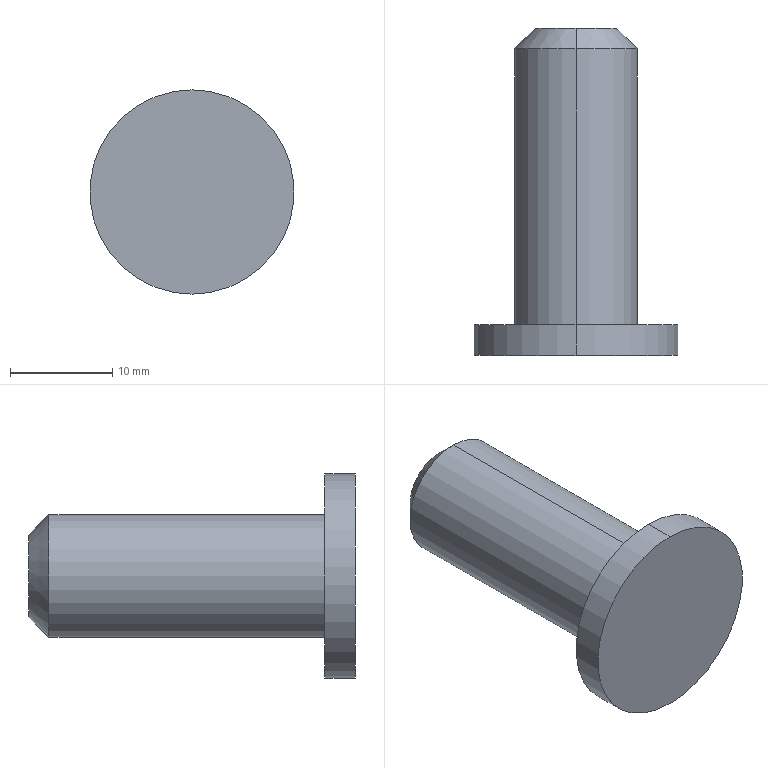Part | SolidWorks | features Chamfer 1, Revolution 1 | 1 solid | 9 faces | box 20 x 32 x 20 mm | volume 4155 mm3 | cylinder 4 | plane 3 | cone 2 | commonest cylinder face diameters 12 x2 20 x2
STEP:
#1=CARTESIAN_POINT('',(0.,32.,4.));
#2=VERTEX_POINT('',#1);
#3=CARTESIAN_POINT('',(0.,32.,-4.));
#4=VERTEX_POINT('',#3);
#5=CARTESIAN_POINT('',(0.,32.,0.));
#6=DIRECTION('',(0.,1.,0.));
#7=DIRECTION('',(0.,0.,1.));
#8=AXIS2_PLACEMENT_3D('',#5,#6,#7);
#9=CIRCLE('',#8,4.);
#10=EDGE_CURVE('',#2,#4,#9,.T.);
#11=ORIENTED_EDGE('',*,*,#10,.F.);
#12=CARTESIAN_POINT('',(0.,30.,6.));
#13=VERTEX_POINT('',#12);
#14=CARTESIAN_POINT('',(0.,30.,6.));
#15=DIRECTION('',(0.,-0.7071,0.7071));
#16=VECTOR('',#15,1000.);
#17=LINE('',#14,#16);
#18=EDGE_CURVE('',#2,#13,#17,.T.);
#19=ORIENTED_EDGE('',*,*,#18,.T.);
#20=CARTESIAN_POINT('',(0.,30.,-6.));
#21=VERTEX_POINT('',#20);
#22=CARTESIAN_POINT('',(0.,30.,0.));
#23=DIRECTION('',(0.,-1.,0.));
#24=DIRECTION('',(0.,0.,1.));
#25=AXIS2_PLACEMENT_3D('',#22,#23,#24);
#26=CIRCLE('',#25,6.);
#27=EDGE_CURVE('',#21,#13,#26,.T.);
#28=ORIENTED_EDGE('',*,*,#27,.F.);
#29=CARTESIAN_POINT('',(0.,30.,-6.));
#30=DIRECTION('',(0.,-0.7071,-0.7071));
#31=VECTOR('',#30,1000.);
#32=LINE('',#29,#31);
#33=EDGE_CURVE('',#4,#21,#32,.T.);
#34=ORIENTED_EDGE('',*,*,#33,.F.);
#35=EDGE_LOOP('',(#11,#19,#28,#34));
#36=FACE_OUTER_BOUND('',#35,.T.);
#37=CARTESIAN_POINT('',(0.,30.,0.));
#38=DIRECTION('',(0.,-1.,0.));
#39=DIRECTION('',(0.,0.,-1.));
#40=AXIS2_PLACEMENT_3D('',#37,#38,#39);
#41=CONICAL_SURFACE('',#40,6.,0.7854);
#42=ADVANCED_FACE('',(#36),#41,.T.);
#43=ORIENTED_EDGE('',*,*,#27,.T.);
#44=CARTESIAN_POINT('',(0.,3.,6.));
#45=VERTEX_POINT('',#44);
#46=CARTESIAN_POINT('',(0.,0.,6.));
#47=DIRECTION('',(0.,-1.,0.));
#48=VECTOR('',#47,1000.);
#49=LINE('',#46,#48);
#50=EDGE_CURVE('',#13,#45,#49,.T.);
#51=ORIENTED_EDGE('',*,*,#50,.T.);
#52=CARTESIAN_POINT('',(0.,3.,-6.));
#53=VERTEX_POINT('',#52);
#54=CARTESIAN_POINT('',(0.,3.,0.));
#55=DIRECTION('',(0.,-1.,0.));
#56=DIRECTION('',(0.,0.,-1.));
#57=AXIS2_PLACEMENT_3D('',#54,#55,#56);
#58=CIRCLE('',#57,6.);
#59=EDGE_CURVE('',#53,#45,#58,.T.);
#60=ORIENTED_EDGE('',*,*,#59,.F.);
#61=CARTESIAN_POINT('',(0.,0.,-6.));
#62=DIRECTION('',(0.,-1.,0.));
#63=VECTOR('',#62,1000.);
#64=LINE('',#61,#63);
#65=EDGE_CURVE('',#21,#53,#64,.T.);
#66=ORIENTED_EDGE('',*,*,#65,.F.);
#67=EDGE_LOOP('',(#43,#51,#60,#66));
#68=FACE_OUTER_BOUND('',#67,.T.);
#69=CARTESIAN_POINT('',(0.,0.,0.));
#70=DIRECTION('',(0.,-1.,0.));
#71=DIRECTION('',(0.,0.,-1.));
#72=AXIS2_PLACEMENT_3D('',#69,#70,#71);
#73=CYLINDRICAL_SURFACE('',#72,6.);
#74=ADVANCED_FACE('',(#68),#73,.T.);
#75=CARTESIAN_POINT('',(0.,3.,-10.));
#76=VERTEX_POINT('',#75);
#77=CARTESIAN_POINT('',(0.,3.,10.));
#78=VERTEX_POINT('',#77);
#79=CARTESIAN_POINT('',(0.,3.,0.));
#80=DIRECTION('',(0.,-1.,0.));
#81=DIRECTION('',(0.,0.,-1.));
#82=AXIS2_PLACEMENT_3D('',#79,#80,#81);
#83=CIRCLE('',#82,10.);
#84=EDGE_CURVE('',#76,#78,#83,.T.);
#85=ORIENTED_EDGE('',*,*,#84,.T.);
#86=CARTESIAN_POINT('',(0.,0.,10.));
#87=VERTEX_POINT('',#86);
#88=CARTESIAN_POINT('',(0.,0.,10.));
#89=DIRECTION('',(0.,-1.,0.));
#90=VECTOR('',#89,1000.);
#91=LINE('',#88,#90);
#92=EDGE_CURVE('',#78,#87,#91,.T.);
#93=ORIENTED_EDGE('',*,*,#92,.T.);
#94=CARTESIAN_POINT('',(0.,0.,-10.));
#95=VERTEX_POINT('',#94);
#96=CARTESIAN_POINT('',(0.,0.,0.));
#97=DIRECTION('',(0.,-1.,0.));
#98=DIRECTION('',(0.,0.,-1.));
#99=AXIS2_PLACEMENT_3D('',#96,#97,#98);
#100=CIRCLE('',#99,10.);
#101=EDGE_CURVE('',#95,#87,#100,.T.);
#102=ORIENTED_EDGE('',*,*,#101,.F.);
#103=CARTESIAN_POINT('',(0.,0.,-10.));
#104=DIRECTION('',(0.,-1.,0.));
#105=VECTOR('',#104,1000.);
#106=LINE('',#103,#105);
#107=EDGE_CURVE('',#76,#95,#106,.T.);
#108=ORIENTED_EDGE('',*,*,#107,.F.);
#109=EDGE_LOOP('',(#85,#93,#102,#108));
#110=FACE_OUTER_BOUND('',#109,.T.);
#111=CARTESIAN_POINT('',(0.,0.,0.));
#112=DIRECTION('',(0.,-1.,0.));
#113=DIRECTION('',(0.,0.,-1.));
#114=AXIS2_PLACEMENT_3D('',#111,#112,#113);
#115=CYLINDRICAL_SURFACE('',#114,10.);
#116=ADVANCED_FACE('',(#110),#115,.T.);
#117=ORIENTED_EDGE('',*,*,#101,.T.);
#118=CARTESIAN_POINT('',(0.,0.,0.));
#119=DIRECTION('',(0.,-1.,0.));
#120=DIRECTION('',(0.,0.,-1.));
#121=AXIS2_PLACEMENT_3D('',#118,#119,#120);
#122=CIRCLE('',#121,10.);
#123=EDGE_CURVE('',#87,#95,#122,.T.);
#124=ORIENTED_EDGE('',*,*,#123,.T.);
#125=EDGE_LOOP('',(#117,#124));
#126=FACE_OUTER_BOUND('',#125,.T.);
#127=CARTESIAN_POINT('',(0.,0.,0.));
#128=DIRECTION('',(0.,-1.,0.));
#129=DIRECTION('',(0.,0.,-1.));
#130=AXIS2_PLACEMENT_3D('',#127,#128,#129);
#131=PLANE('',#130);
#132=ADVANCED_FACE('',(#126),#131,.T.);
#133=ORIENTED_EDGE('',*,*,#92,.F.);
#134=CARTESIAN_POINT('',(0.,3.,0.));
#135=DIRECTION('',(0.,-1.,0.));
#136=DIRECTION('',(0.,0.,-1.));
#137=AXIS2_PLACEMENT_3D('',#134,#135,#136);
#138=CIRCLE('',#137,10.);
#139=EDGE_CURVE('',#78,#76,#138,.T.);
#140=ORIENTED_EDGE('',*,*,#139,.T.);
#141=ORIENTED_EDGE('',*,*,#107,.T.);
#142=ORIENTED_EDGE('',*,*,#123,.F.);
#143=EDGE_LOOP('',(#133,#140,#141,#142));
#144=FACE_OUTER_BOUND('',#143,.T.);
#145=CARTESIAN_POINT('',(0.,0.,0.));
#146=DIRECTION('',(0.,-1.,0.));
#147=DIRECTION('',(0.,0.,-1.));
#148=AXIS2_PLACEMENT_3D('',#145,#146,#147);
#149=CYLINDRICAL_SURFACE('',#148,10.);
#150=ADVANCED_FACE('',(#144),#149,.T.);
#151=ORIENTED_EDGE('',*,*,#59,.T.);
#152=CARTESIAN_POINT('',(0.,3.,0.));
#153=DIRECTION('',(0.,-1.,0.));
#154=DIRECTION('',(0.,0.,-1.));
#155=AXIS2_PLACEMENT_3D('',#152,#153,#154);
#156=CIRCLE('',#155,6.);
#157=EDGE_CURVE('',#45,#53,#156,.T.);
#158=ORIENTED_EDGE('',*,*,#157,.T.);
#159=EDGE_LOOP('',(#151,#158));
#160=FACE_BOUND('',#159,.T.);
#161=ORIENTED_EDGE('',*,*,#84,.F.);
#162=ORIENTED_EDGE('',*,*,#139,.F.);
#163=EDGE_LOOP('',(#161,#162));
#164=FACE_OUTER_BOUND('',#163,.T.);
#165=CARTESIAN_POINT('',(10.,3.,0.));
#166=DIRECTION('',(0.,1.,0.));
#167=DIRECTION('',(0.,0.,1.));
#168=AXIS2_PLACEMENT_3D('',#165,#166,#167);
#169=PLANE('',#168);
#170=ADVANCED_FACE('',(#160,#164),#169,.T.);
#171=ORIENTED_EDGE('',*,*,#50,.F.);
#172=CARTESIAN_POINT('',(0.,30.,0.));
#173=DIRECTION('',(0.,-1.,0.));
#174=DIRECTION('',(0.,0.,1.));
#175=AXIS2_PLACEMENT_3D('',#172,#173,#174);
#176=CIRCLE('',#175,6.);
#177=EDGE_CURVE('',#13,#21,#176,.T.);
#178=ORIENTED_EDGE('',*,*,#177,.T.);
#179=ORIENTED_EDGE('',*,*,#65,.T.);
#180=ORIENTED_EDGE('',*,*,#157,.F.);
#181=EDGE_LOOP('',(#171,#178,#179,#180));
#182=FACE_OUTER_BOUND('',#181,.T.);
#183=CARTESIAN_POINT('',(0.,0.,0.));
#184=DIRECTION('',(0.,-1.,0.));
#185=DIRECTION('',(0.,0.,-1.));
#186=AXIS2_PLACEMENT_3D('',#183,#184,#185);
#187=CYLINDRICAL_SURFACE('',#186,6.);
#188=ADVANCED_FACE('',(#182),#187,.T.);
#189=CARTESIAN_POINT('',(0.,32.,0.));
#190=DIRECTION('',(0.,1.,0.));
#191=DIRECTION('',(0.,0.,1.));
#192=AXIS2_PLACEMENT_3D('',#189,#190,#191);
#193=CIRCLE('',#192,4.);
#194=EDGE_CURVE('',#4,#2,#193,.T.);
#195=ORIENTED_EDGE('',*,*,#194,.T.);
#196=ORIENTED_EDGE('',*,*,#10,.T.);
#197=EDGE_LOOP('',(#195,#196));
#198=FACE_OUTER_BOUND('',#197,.T.);
#199=CARTESIAN_POINT('',(6.,32.,0.));
#200=DIRECTION('',(0.,1.,0.));
#201=DIRECTION('',(0.,0.,1.));
#202=AXIS2_PLACEMENT_3D('',#199,#200,#201);
#203=PLANE('',#202);
#204=ADVANCED_FACE('',(#198),#203,.T.);
#205=ORIENTED_EDGE('',*,*,#18,.F.);
#206=ORIENTED_EDGE('',*,*,#194,.F.);
#207=ORIENTED_EDGE('',*,*,#33,.T.);
#208=ORIENTED_EDGE('',*,*,#177,.F.);
#209=EDGE_LOOP('',(#205,#206,#207,#208));
#210=FACE_OUTER_BOUND('',#209,.T.);
#211=CARTESIAN_POINT('',(0.,30.,0.));
#212=DIRECTION('',(0.,-1.,0.));
#213=DIRECTION('',(0.,0.,-1.));
#214=AXIS2_PLACEMENT_3D('',#211,#212,#213);
#215=CONICAL_SURFACE('',#214,6.,0.7854);
#216=ADVANCED_FACE('',(#210),#215,.T.);
#217=CLOSED_SHELL('',(#42,#74,#116,#132,#150,#170,#188,#204,#216));
#218=MANIFOLD_SOLID_BREP('',#217);
#219=CARTESIAN_POINT('',(0.,0.,0.));
#220=DIRECTION('',(0.,0.,1.));
#221=DIRECTION('',(1.,0.,0.));
#222=AXIS2_PLACEMENT_3D('',#219,#220,#221);
#223=(LENGTH_UNIT()NAMED_UNIT(*)SI_UNIT(.MILLI.,.METRE.));
#224=UNCERTAINTY_MEASURE_WITH_UNIT(LENGTH_MEASURE(0.00001),#223,'','');
#225=(NAMED_UNIT(*)PLANE_ANGLE_UNIT()SI_UNIT($,.RADIAN.));
#226=(NAMED_UNIT(*)SI_UNIT($,.STERADIAN.)SOLID_ANGLE_UNIT());
#227=(GEOMETRIC_REPRESENTATION_CONTEXT(3)GLOBAL_UNCERTAINTY_ASSIGNED_CONTEXT((#224))GLOBAL_UNIT_ASSIGNED_CONTEXT((#223,#225,#226))REPRESENTATION_CONTEXT('',''));
#228=ADVANCED_BREP_SHAPE_REPRESENTATION('',(#218,#222),#227);